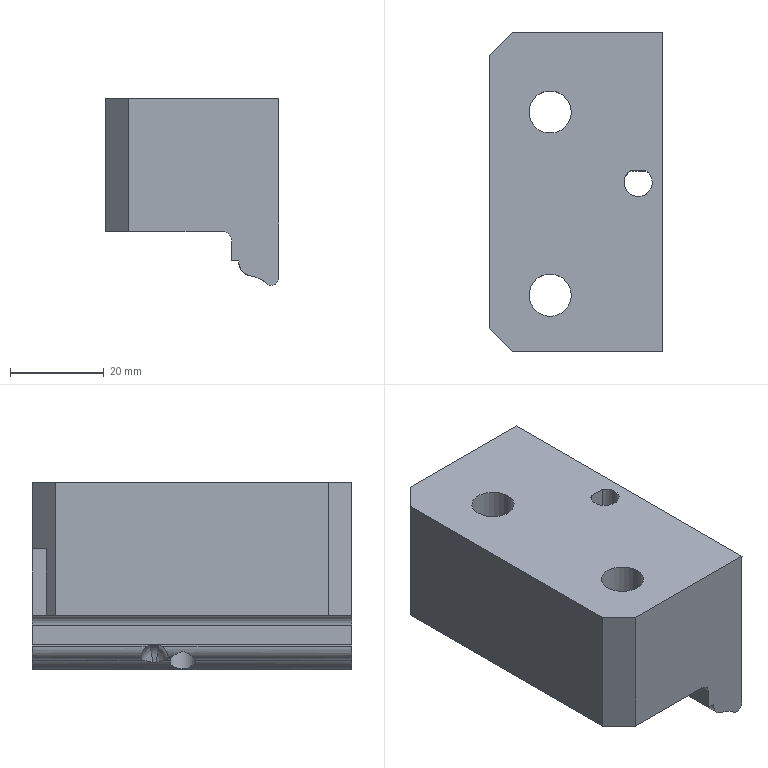Part | 1 solid | 37 faces | box 37.011 x 68 x 39.792 mm | volume 68619 mm3 | plane 19 | cylinder 15 | spline 3 | commonest cylinder face diameters 9 x4 16 x4 6.4 x2 11.371 x2 3.1 x1 4 x1